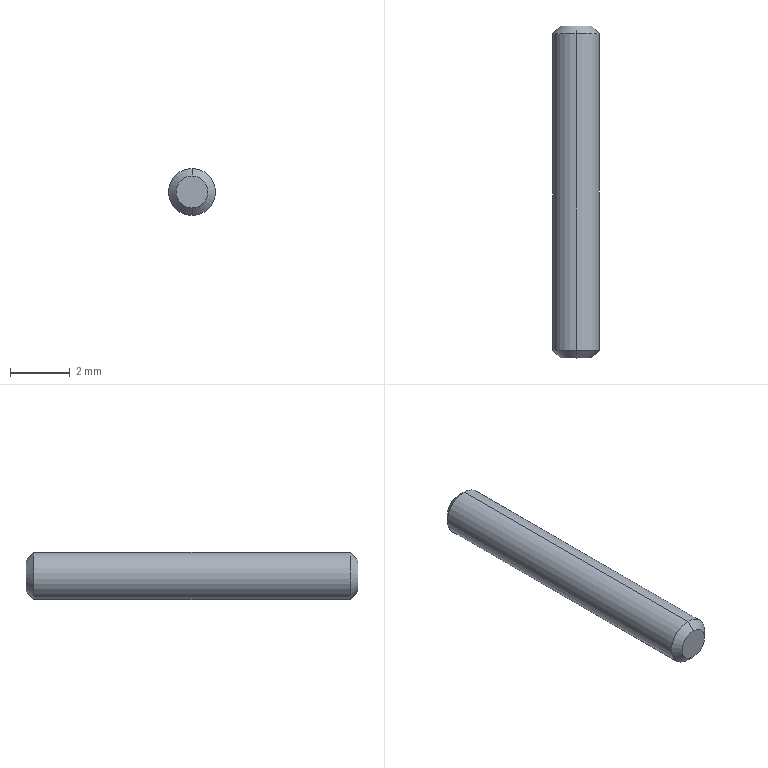Part | SolidWorks | features Chamfer 1, Extrusion 1 | 1 solid | 8 faces | box 1.575 x 11.112 x 1.575 mm | volume 21.36 mm3 | cone 4 | cylinder 2 | plane 2 | commonest cylinder face diameters 1.575 x2
STEP:
#1=CARTESIAN_POINT('',(0.,0.,-0.021));
#2=VERTEX_POINT('',#1);
#3=CARTESIAN_POINT('',(0.,0.,0.021));
#4=VERTEX_POINT('',#3);
#5=CARTESIAN_POINT('',(0.,0.,0.));
#6=DIRECTION('',(0.,-1.,0.));
#7=DIRECTION('',(0.,0.,1.));
#8=AXIS2_PLACEMENT_3D('',#5,#6,#7);
#9=CIRCLE('',#8,0.021);
#10=EDGE_CURVE('',#2,#4,#9,.T.);
#11=ORIENTED_EDGE('',*,*,#10,.F.);
#12=CARTESIAN_POINT('',(0.,0.01,-0.031));
#13=VERTEX_POINT('',#12);
#14=CARTESIAN_POINT('',(0.,0.01,-0.031));
#15=DIRECTION('',(0.,0.7071,-0.7071));
#16=VECTOR('',#15,39.37);
#17=LINE('',#14,#16);
#18=EDGE_CURVE('',#2,#13,#17,.T.);
#19=ORIENTED_EDGE('',*,*,#18,.T.);
#20=CARTESIAN_POINT('',(0.,0.01,0.031));
#21=VERTEX_POINT('',#20);
#22=CARTESIAN_POINT('',(0.,0.01,0.));
#23=DIRECTION('',(0.,1.,0.));
#24=DIRECTION('',(0.,0.,1.));
#25=AXIS2_PLACEMENT_3D('',#22,#23,#24);
#26=CIRCLE('',#25,0.031);
#27=EDGE_CURVE('',#21,#13,#26,.T.);
#28=ORIENTED_EDGE('',*,*,#27,.F.);
#29=CARTESIAN_POINT('',(0.,0.01,0.031));
#30=DIRECTION('',(0.,0.7071,0.7071));
#31=VECTOR('',#30,39.37);
#32=LINE('',#29,#31);
#33=EDGE_CURVE('',#4,#21,#32,.T.);
#34=ORIENTED_EDGE('',*,*,#33,.F.);
#35=EDGE_LOOP('',(#11,#19,#28,#34));
#36=FACE_OUTER_BOUND('',#35,.T.);
#37=CARTESIAN_POINT('',(0.,0.01,0.));
#38=DIRECTION('',(0.,1.,0.));
#39=DIRECTION('',(0.,0.,1.));
#40=AXIS2_PLACEMENT_3D('',#37,#38,#39);
#41=CONICAL_SURFACE('',#40,0.031,0.7854);
#42=ADVANCED_FACE('',(#36),#41,.T.);
#43=CARTESIAN_POINT('',(0.,0.4375,0.021));
#44=VERTEX_POINT('',#43);
#45=CARTESIAN_POINT('',(0.,0.4375,-0.021));
#46=VERTEX_POINT('',#45);
#47=CARTESIAN_POINT('',(0.,0.4375,0.));
#48=DIRECTION('',(0.,1.,0.));
#49=DIRECTION('',(0.,0.,1.));
#50=AXIS2_PLACEMENT_3D('',#47,#48,#49);
#51=CIRCLE('',#50,0.021);
#52=EDGE_CURVE('',#44,#46,#51,.T.);
#53=ORIENTED_EDGE('',*,*,#52,.F.);
#54=CARTESIAN_POINT('',(0.,0.4275,0.031));
#55=VERTEX_POINT('',#54);
#56=CARTESIAN_POINT('',(0.,0.4375,0.021));
#57=DIRECTION('',(0.,-0.7071,0.7071));
#58=VECTOR('',#57,39.37);
#59=LINE('',#56,#58);
#60=EDGE_CURVE('',#44,#55,#59,.T.);
#61=ORIENTED_EDGE('',*,*,#60,.T.);
#62=CARTESIAN_POINT('',(0.,0.4275,-0.031));
#63=VERTEX_POINT('',#62);
#64=CARTESIAN_POINT('',(0.,0.4275,0.));
#65=DIRECTION('',(0.,-1.,0.));
#66=DIRECTION('',(0.,0.,1.));
#67=AXIS2_PLACEMENT_3D('',#64,#65,#66);
#68=CIRCLE('',#67,0.031);
#69=EDGE_CURVE('',#63,#55,#68,.T.);
#70=ORIENTED_EDGE('',*,*,#69,.F.);
#71=CARTESIAN_POINT('',(0.,0.4375,-0.021));
#72=DIRECTION('',(0.,-0.7071,-0.7071));
#73=VECTOR('',#72,39.37);
#74=LINE('',#71,#73);
#75=EDGE_CURVE('',#46,#63,#74,.T.);
#76=ORIENTED_EDGE('',*,*,#75,.F.);
#77=EDGE_LOOP('',(#53,#61,#70,#76));
#78=FACE_OUTER_BOUND('',#77,.T.);
#79=CARTESIAN_POINT('',(0.,0.4375,0.));
#80=DIRECTION('',(0.,-1.,0.));
#81=DIRECTION('',(0.,0.,-1.));
#82=AXIS2_PLACEMENT_3D('',#79,#80,#81);
#83=CONICAL_SURFACE('',#82,0.021,0.7854);
#84=ADVANCED_FACE('',(#78),#83,.T.);
#85=ORIENTED_EDGE('',*,*,#69,.T.);
#86=CARTESIAN_POINT('',(0.,0.4375,0.031));
#87=DIRECTION('',(0.,-1.,0.));
#88=VECTOR('',#87,39.37);
#89=LINE('',#86,#88);
#90=EDGE_CURVE('',#55,#21,#89,.T.);
#91=ORIENTED_EDGE('',*,*,#90,.T.);
#92=ORIENTED_EDGE('',*,*,#27,.T.);
#93=CARTESIAN_POINT('',(0.,0.4375,-0.031));
#94=DIRECTION('',(0.,-1.,0.));
#95=VECTOR('',#94,39.37);
#96=LINE('',#93,#95);
#97=EDGE_CURVE('',#63,#13,#96,.T.);
#98=ORIENTED_EDGE('',*,*,#97,.F.);
#99=EDGE_LOOP('',(#85,#91,#92,#98));
#100=FACE_OUTER_BOUND('',#99,.T.);
#101=CARTESIAN_POINT('',(0.,0.4375,0.));
#102=DIRECTION('',(0.,-1.,0.));
#103=DIRECTION('',(0.,0.,-1.));
#104=AXIS2_PLACEMENT_3D('',#101,#102,#103);
#105=CYLINDRICAL_SURFACE('',#104,0.031);
#106=ADVANCED_FACE('',(#100),#105,.T.);
#107=ORIENTED_EDGE('',*,*,#90,.F.);
#108=CARTESIAN_POINT('',(0.,0.4275,0.));
#109=DIRECTION('',(0.,-1.,0.));
#110=DIRECTION('',(0.,0.,1.));
#111=AXIS2_PLACEMENT_3D('',#108,#109,#110);
#112=CIRCLE('',#111,0.031);
#113=EDGE_CURVE('',#55,#63,#112,.T.);
#114=ORIENTED_EDGE('',*,*,#113,.T.);
#115=ORIENTED_EDGE('',*,*,#97,.T.);
#116=CARTESIAN_POINT('',(0.,0.01,0.));
#117=DIRECTION('',(0.,1.,0.));
#118=DIRECTION('',(0.,0.,1.));
#119=AXIS2_PLACEMENT_3D('',#116,#117,#118);
#120=CIRCLE('',#119,0.031);
#121=EDGE_CURVE('',#13,#21,#120,.T.);
#122=ORIENTED_EDGE('',*,*,#121,.T.);
#123=EDGE_LOOP('',(#107,#114,#115,#122));
#124=FACE_OUTER_BOUND('',#123,.T.);
#125=CARTESIAN_POINT('',(0.,0.4375,0.));
#126=DIRECTION('',(0.,-1.,0.));
#127=DIRECTION('',(0.,0.,-1.));
#128=AXIS2_PLACEMENT_3D('',#125,#126,#127);
#129=CYLINDRICAL_SURFACE('',#128,0.031);
#130=ADVANCED_FACE('',(#124),#129,.T.);
#131=CARTESIAN_POINT('',(0.,0.4375,0.));
#132=DIRECTION('',(0.,1.,0.));
#133=DIRECTION('',(0.,0.,1.));
#134=AXIS2_PLACEMENT_3D('',#131,#132,#133);
#135=CIRCLE('',#134,0.021);
#136=EDGE_CURVE('',#46,#44,#135,.T.);
#137=ORIENTED_EDGE('',*,*,#136,.T.);
#138=ORIENTED_EDGE('',*,*,#52,.T.);
#139=EDGE_LOOP('',(#137,#138));
#140=FACE_OUTER_BOUND('',#139,.T.);
#141=CARTESIAN_POINT('',(0.,0.4375,0.));
#142=DIRECTION('',(0.,1.,0.));
#143=DIRECTION('',(0.,0.,1.));
#144=AXIS2_PLACEMENT_3D('',#141,#142,#143);
#145=PLANE('',#144);
#146=ADVANCED_FACE('',(#140),#145,.T.);
#147=CARTESIAN_POINT('',(0.,0.,0.));
#148=DIRECTION('',(0.,-1.,0.));
#149=DIRECTION('',(0.,0.,1.));
#150=AXIS2_PLACEMENT_3D('',#147,#148,#149);
#151=CIRCLE('',#150,0.021);
#152=EDGE_CURVE('',#4,#2,#151,.T.);
#153=ORIENTED_EDGE('',*,*,#152,.T.);
#154=ORIENTED_EDGE('',*,*,#10,.T.);
#155=EDGE_LOOP('',(#153,#154));
#156=FACE_OUTER_BOUND('',#155,.T.);
#157=CARTESIAN_POINT('',(0.,0.,0.));
#158=DIRECTION('',(0.,1.,0.));
#159=DIRECTION('',(0.,0.,1.));
#160=AXIS2_PLACEMENT_3D('',#157,#158,#159);
#161=PLANE('',#160);
#162=ADVANCED_FACE('',(#156),#161,.F.);
#163=ORIENTED_EDGE('',*,*,#60,.F.);
#164=ORIENTED_EDGE('',*,*,#136,.F.);
#165=ORIENTED_EDGE('',*,*,#75,.T.);
#166=ORIENTED_EDGE('',*,*,#113,.F.);
#167=EDGE_LOOP('',(#163,#164,#165,#166));
#168=FACE_OUTER_BOUND('',#167,.T.);
#169=CARTESIAN_POINT('',(0.,0.4375,0.));
#170=DIRECTION('',(0.,-1.,0.));
#171=DIRECTION('',(0.,0.,-1.));
#172=AXIS2_PLACEMENT_3D('',#169,#170,#171);
#173=CONICAL_SURFACE('',#172,0.021,0.7854);
#174=ADVANCED_FACE('',(#168),#173,.T.);
#175=ORIENTED_EDGE('',*,*,#18,.F.);
#176=ORIENTED_EDGE('',*,*,#152,.F.);
#177=ORIENTED_EDGE('',*,*,#33,.T.);
#178=ORIENTED_EDGE('',*,*,#121,.F.);
#179=EDGE_LOOP('',(#175,#176,#177,#178));
#180=FACE_OUTER_BOUND('',#179,.T.);
#181=CARTESIAN_POINT('',(0.,0.01,0.));
#182=DIRECTION('',(0.,1.,0.));
#183=DIRECTION('',(0.,0.,1.));
#184=AXIS2_PLACEMENT_3D('',#181,#182,#183);
#185=CONICAL_SURFACE('',#184,0.031,0.7854);
#186=ADVANCED_FACE('',(#180),#185,.T.);
#187=CLOSED_SHELL('',(#42,#84,#106,#130,#146,#162,#174,#186));
#188=MANIFOLD_SOLID_BREP('',#187);
#189=CARTESIAN_POINT('',(0.,0.,0.));
#190=DIRECTION('',(0.,0.,1.));
#191=DIRECTION('',(1.,0.,0.));
#192=AXIS2_PLACEMENT_3D('',#189,#190,#191);
#193=(LENGTH_UNIT()NAMED_UNIT(*)SI_UNIT($,.METRE.));
#194=LENGTH_MEASURE_WITH_UNIT(LENGTH_MEASURE(0.0254),#193);
#195=DIMENSIONAL_EXPONENTS(1.,0.,0.,0.,0.,0.,0.);
#196=(CONVERSION_BASED_UNIT('INCH',#194)LENGTH_UNIT()NAMED_UNIT(#195));
#197=UNCERTAINTY_MEASURE_WITH_UNIT(LENGTH_MEASURE(0.00001),#196,'','');
#198=(NAMED_UNIT(*)PLANE_ANGLE_UNIT()SI_UNIT($,.RADIAN.));
#199=(NAMED_UNIT(*)SI_UNIT($,.STERADIAN.)SOLID_ANGLE_UNIT());
#200=(GEOMETRIC_REPRESENTATION_CONTEXT(3)GLOBAL_UNCERTAINTY_ASSIGNED_CONTEXT((#197))GLOBAL_UNIT_ASSIGNED_CONTEXT((#196,#198,#199))REPRESENTATION_CONTEXT('',''));
#201=ADVANCED_BREP_SHAPE_REPRESENTATION('',(#188,#192),#200);